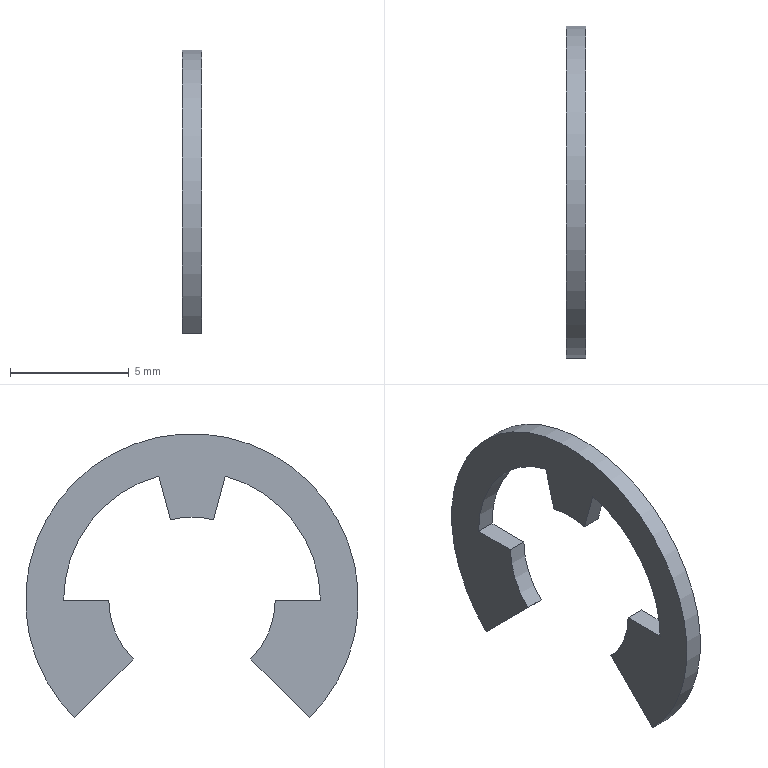Part | STEP file | 0217_Z_SCCG8-55-2 | 1 solid | 14 faces | box 0.8 x 14 x 11.95 mm | volume 51.564 mm3 | plane 8 | cylinder 6 | commonest cylinder face diameters 7 x3 10.8 x2 14 x1
STEP:
#1=CARTESIAN_POINT('',(0.,0.,0.));
#2=DIRECTION('',(0.,0.,1.));
#3=DIRECTION('',(1.,0.,0.));
#4=AXIS2_PLACEMENT_3D('',#1,#2,#3);
#5=CARTESIAN_POINT('',(3.,-2.475,-2.475));
#6=VERTEX_POINT('',#5);
#7=CARTESIAN_POINT('',(3.,-4.95,-4.95));
#8=VERTEX_POINT('',#7);
#9=CARTESIAN_POINT('',(3.,-2.475,-2.475));
#10=DIRECTION('',(0.,-0.7071,-0.7071));
#11=VECTOR('',#10,1.);
#12=LINE('',#9,#11);
#13=CARTESIAN_POINT('',(3.,0.,0.));
#14=DIRECTION('',(-1.,0.,0.));
#15=DIRECTION('',(0.,0.,1.));
#16=AXIS2_PLACEMENT_3D('',#13,#14,#15);
#17=PLANE('',#16);
#18=CARTESIAN_POINT('',(-2.475,-2.475));
#19=DIRECTION('',(-0.7071,-0.7071));
#20=VECTOR('',#19,1.);
#21=LINE('',#18,#20);
#22=(GEOMETRIC_REPRESENTATION_CONTEXT(2)PARAMETRIC_REPRESENTATION_CONTEXT()REPRESENTATION_CONTEXT('',''));
#23=DEFINITIONAL_REPRESENTATION('',(#21),#22);
#24=PCURVE('',#17,#23);
#25=CARTESIAN_POINT('',(3.,-4.95,-4.95));
#26=DIRECTION('',(0.,0.7071,-0.7071));
#27=DIRECTION('',(0.,0.7071,0.7071));
#28=AXIS2_PLACEMENT_3D('',#25,#26,#27);
#29=PLANE('',#28);
#30=CARTESIAN_POINT('',(3.5,0.));
#31=DIRECTION('',(-1.,0.));
#32=VECTOR('',#31,1.);
#33=LINE('',#30,#32);
#34=(GEOMETRIC_REPRESENTATION_CONTEXT(2)PARAMETRIC_REPRESENTATION_CONTEXT()REPRESENTATION_CONTEXT('',''));
#35=DEFINITIONAL_REPRESENTATION('',(#33),#34);
#36=PCURVE('',#29,#35);
#37=SURFACE_CURVE('',#12,(#24,#36),.PCURVE_S1.);
#38=EDGE_CURVE('',#6,#8,#37,.T.);
#39=ORIENTED_EDGE('',*,*,#38,.F.);
#40=CARTESIAN_POINT('',(3.,-3.5,0.));
#41=VERTEX_POINT('',#40);
#42=CARTESIAN_POINT('',(3.,0.,0.));
#43=DIRECTION('',(1.,0.,0.));
#44=DIRECTION('',(0.,0.,-1.));
#45=AXIS2_PLACEMENT_3D('',#42,#43,#44);
#46=CIRCLE('',#45,3.5);
#47=CARTESIAN_POINT('',(-3.5,0.));
#48=CARTESIAN_POINT('',(-3.5,6.062));
#49=CARTESIAN_POINT('',(1.75,3.031));
#50=CARTESIAN_POINT('',(7.,0.));
#51=CARTESIAN_POINT('',(1.75,-3.031));
#52=CARTESIAN_POINT('',(-3.5,-6.062));
#53=CARTESIAN_POINT('',(-3.5,0.));
#54=(BOUNDED_CURVE()B_SPLINE_CURVE(2,(#47,#48,#49,#50,#51,#52,#53),.UNSPECIFIED.,.T.,.F.)B_SPLINE_CURVE_WITH_KNOTS((1,2,2,2,2,1),(-2.094,0.,2.094,4.189,6.283,8.378),.UNSPECIFIED.)CURVE()GEOMETRIC_REPRESENTATION_ITEM()RATIONAL_B_SPLINE_CURVE((1.,0.5,1.,0.5,1.,0.5,1.))REPRESENTATION_ITEM(''));
#55=(GEOMETRIC_REPRESENTATION_CONTEXT(2)PARAMETRIC_REPRESENTATION_CONTEXT()REPRESENTATION_CONTEXT('',''));
#56=DEFINITIONAL_REPRESENTATION('',(#54),#55);
#57=PCURVE('',#17,#56);
#58=CARTESIAN_POINT('',(3.,0.,0.));
#59=DIRECTION('',(1.,0.,0.));
#60=DIRECTION('',(0.,0.,-1.));
#61=AXIS2_PLACEMENT_3D('',#58,#59,#60);
#62=CYLINDRICAL_SURFACE('',#61,3.5);
#63=CARTESIAN_POINT('',(0.,0.));
#64=DIRECTION('',(1.,0.));
#65=VECTOR('',#64,1.);
#66=LINE('',#63,#65);
#67=(GEOMETRIC_REPRESENTATION_CONTEXT(2)PARAMETRIC_REPRESENTATION_CONTEXT()REPRESENTATION_CONTEXT('',''));
#68=DEFINITIONAL_REPRESENTATION('',(#66),#67);
#69=PCURVE('',#62,#68);
#70=SURFACE_CURVE('',#46,(#57,#69),.PCURVE_S1.);
#71=EDGE_CURVE('',#41,#6,#70,.T.);
#72=ORIENTED_EDGE('',*,*,#71,.F.);
#73=CARTESIAN_POINT('',(3.,-5.4,0.));
#74=VERTEX_POINT('',#73);
#75=CARTESIAN_POINT('',(3.,0.,0.));
#76=DIRECTION('',(0.,1.,0.));
#77=VECTOR('',#76,1.);
#78=LINE('',#75,#77);
#79=CARTESIAN_POINT('',(0.,0.));
#80=DIRECTION('',(0.,1.));
#81=VECTOR('',#80,1.);
#82=LINE('',#79,#81);
#83=(GEOMETRIC_REPRESENTATION_CONTEXT(2)PARAMETRIC_REPRESENTATION_CONTEXT()REPRESENTATION_CONTEXT('',''));
#84=DEFINITIONAL_REPRESENTATION('',(#82),#83);
#85=PCURVE('',#17,#84);
#86=CARTESIAN_POINT('',(3.,-3.5,0.));
#87=DIRECTION('',(0.,0.,1.));
#88=DIRECTION('',(1.,0.,0.));
#89=AXIS2_PLACEMENT_3D('',#86,#87,#88);
#90=PLANE('',#89);
#91=CARTESIAN_POINT('',(0.,3.5));
#92=DIRECTION('',(0.,1.));
#93=VECTOR('',#92,1.);
#94=LINE('',#91,#93);
#95=(GEOMETRIC_REPRESENTATION_CONTEXT(2)PARAMETRIC_REPRESENTATION_CONTEXT()REPRESENTATION_CONTEXT('',''));
#96=DEFINITIONAL_REPRESENTATION('',(#94),#95);
#97=PCURVE('',#90,#96);
#98=SURFACE_CURVE('',#78,(#85,#97),.PCURVE_S1.);
#99=EDGE_CURVE('',#74,#41,#98,.T.);
#100=ORIENTED_EDGE('',*,*,#99,.F.);
#101=CARTESIAN_POINT('',(3.,-1.398,5.216));
#102=VERTEX_POINT('',#101);
#103=CARTESIAN_POINT('',(3.,0.,0.));
#104=DIRECTION('',(1.,0.,0.));
#105=DIRECTION('',(0.,0.,-1.));
#106=AXIS2_PLACEMENT_3D('',#103,#104,#105);
#107=CIRCLE('',#106,5.4);
#108=CARTESIAN_POINT('',(-5.4,0.));
#109=CARTESIAN_POINT('',(-5.4,9.353));
#110=CARTESIAN_POINT('',(2.7,4.677));
#111=CARTESIAN_POINT('',(10.8,0.));
#112=CARTESIAN_POINT('',(2.7,-4.677));
#113=CARTESIAN_POINT('',(-5.4,-9.353));
#114=CARTESIAN_POINT('',(-5.4,0.));
#115=(BOUNDED_CURVE()B_SPLINE_CURVE(2,(#108,#109,#110,#111,#112,#113,#114),.UNSPECIFIED.,.T.,.F.)B_SPLINE_CURVE_WITH_KNOTS((1,2,2,2,2,1),(-2.094,0.,2.094,4.189,6.283,8.378),.UNSPECIFIED.)CURVE()GEOMETRIC_REPRESENTATION_ITEM()RATIONAL_B_SPLINE_CURVE((1.,0.5,1.,0.5,1.,0.5,1.))REPRESENTATION_ITEM(''));
#116=(GEOMETRIC_REPRESENTATION_CONTEXT(2)PARAMETRIC_REPRESENTATION_CONTEXT()REPRESENTATION_CONTEXT('',''));
#117=DEFINITIONAL_REPRESENTATION('',(#115),#116);
#118=PCURVE('',#17,#117);
#119=CARTESIAN_POINT('',(3.,0.,0.));
#120=DIRECTION('',(1.,0.,0.));
#121=DIRECTION('',(0.,0.,-1.));
#122=AXIS2_PLACEMENT_3D('',#119,#120,#121);
#123=CYLINDRICAL_SURFACE('',#122,5.4);
#124=CARTESIAN_POINT('',(0.,0.));
#125=DIRECTION('',(1.,0.));
#126=VECTOR('',#125,1.);
#127=LINE('',#124,#126);
#128=(GEOMETRIC_REPRESENTATION_CONTEXT(2)PARAMETRIC_REPRESENTATION_CONTEXT()REPRESENTATION_CONTEXT('',''));
#129=DEFINITIONAL_REPRESENTATION('',(#127),#128);
#130=PCURVE('',#123,#129);
#131=SURFACE_CURVE('',#107,(#118,#130),.PCURVE_S1.);
#132=EDGE_CURVE('',#102,#74,#131,.T.);
#133=ORIENTED_EDGE('',*,*,#132,.F.);
#134=CARTESIAN_POINT('',(3.,-0.9059,3.381));
#135=VERTEX_POINT('',#134);
#136=CARTESIAN_POINT('',(3.,-0.9059,3.381));
#137=DIRECTION('',(0.,-0.2588,0.9659));
#138=VECTOR('',#137,1.);
#139=LINE('',#136,#138);
#140=CARTESIAN_POINT('',(3.381,-0.9059));
#141=DIRECTION('',(0.9659,-0.2588));
#142=VECTOR('',#141,1.);
#143=LINE('',#140,#142);
#144=(GEOMETRIC_REPRESENTATION_CONTEXT(2)PARAMETRIC_REPRESENTATION_CONTEXT()REPRESENTATION_CONTEXT('',''));
#145=DEFINITIONAL_REPRESENTATION('',(#143),#144);
#146=PCURVE('',#17,#145);
#147=CARTESIAN_POINT('',(3.,-1.398,5.216));
#148=DIRECTION('',(0.,-0.9659,-0.2588));
#149=DIRECTION('',(0.,0.2588,-0.9659));
#150=AXIS2_PLACEMENT_3D('',#147,#148,#149);
#151=PLANE('',#150);
#152=CARTESIAN_POINT('',(1.9,0.));
#153=DIRECTION('',(-1.,0.));
#154=VECTOR('',#153,1.);
#155=LINE('',#152,#154);
#156=(GEOMETRIC_REPRESENTATION_CONTEXT(2)PARAMETRIC_REPRESENTATION_CONTEXT()REPRESENTATION_CONTEXT('',''));
#157=DEFINITIONAL_REPRESENTATION('',(#155),#156);
#158=PCURVE('',#151,#157);
#159=SURFACE_CURVE('',#139,(#146,#158),.PCURVE_S1.);
#160=EDGE_CURVE('',#135,#102,#159,.T.);
#161=ORIENTED_EDGE('',*,*,#160,.F.);
#162=CARTESIAN_POINT('',(3.,0.9059,3.381));
#163=VERTEX_POINT('',#162);
#164=CARTESIAN_POINT('',(3.,0.,0.));
#165=DIRECTION('',(1.,0.,0.));
#166=DIRECTION('',(0.,0.,-1.));
#167=AXIS2_PLACEMENT_3D('',#164,#165,#166);
#168=CIRCLE('',#167,3.5);
#169=CARTESIAN_POINT('',(-3.5,0.));
#170=CARTESIAN_POINT('',(-3.5,6.062));
#171=CARTESIAN_POINT('',(1.75,3.031));
#172=CARTESIAN_POINT('',(7.,0.));
#173=CARTESIAN_POINT('',(1.75,-3.031));
#174=CARTESIAN_POINT('',(-3.5,-6.062));
#175=CARTESIAN_POINT('',(-3.5,0.));
#176=(BOUNDED_CURVE()B_SPLINE_CURVE(2,(#169,#170,#171,#172,#173,#174,#175),.UNSPECIFIED.,.T.,.F.)B_SPLINE_CURVE_WITH_KNOTS((1,2,2,2,2,1),(-2.094,0.,2.094,4.189,6.283,8.378),.UNSPECIFIED.)CURVE()GEOMETRIC_REPRESENTATION_ITEM()RATIONAL_B_SPLINE_CURVE((1.,0.5,1.,0.5,1.,0.5,1.))REPRESENTATION_ITEM(''));
#177=(GEOMETRIC_REPRESENTATION_CONTEXT(2)PARAMETRIC_REPRESENTATION_CONTEXT()REPRESENTATION_CONTEXT('',''));
#178=DEFINITIONAL_REPRESENTATION('',(#176),#177);
#179=PCURVE('',#17,#178);
#180=CARTESIAN_POINT('',(3.,0.,0.));
#181=DIRECTION('',(1.,0.,0.));
#182=DIRECTION('',(0.,0.,-1.));
#183=AXIS2_PLACEMENT_3D('',#180,#181,#182);
#184=CYLINDRICAL_SURFACE('',#183,3.5);
#185=CARTESIAN_POINT('',(0.,0.));
#186=DIRECTION('',(1.,0.));
#187=VECTOR('',#186,1.);
#188=LINE('',#185,#187);
#189=(GEOMETRIC_REPRESENTATION_CONTEXT(2)PARAMETRIC_REPRESENTATION_CONTEXT()REPRESENTATION_CONTEXT('',''));
#190=DEFINITIONAL_REPRESENTATION('',(#188),#189);
#191=PCURVE('',#184,#190);
#192=SURFACE_CURVE('',#168,(#179,#191),.PCURVE_S1.);
#193=EDGE_CURVE('',#163,#135,#192,.T.);
#194=ORIENTED_EDGE('',*,*,#193,.F.);
#195=CARTESIAN_POINT('',(3.,1.398,5.216));
#196=VERTEX_POINT('',#195);
#197=CARTESIAN_POINT('',(3.,1.398,5.216));
#198=DIRECTION('',(0.,-0.2588,-0.9659));
#199=VECTOR('',#198,1.);
#200=LINE('',#197,#199);
#201=CARTESIAN_POINT('',(5.216,1.398));
#202=DIRECTION('',(-0.9659,-0.2588));
#203=VECTOR('',#202,1.);
#204=LINE('',#201,#203);
#205=(GEOMETRIC_REPRESENTATION_CONTEXT(2)PARAMETRIC_REPRESENTATION_CONTEXT()REPRESENTATION_CONTEXT('',''));
#206=DEFINITIONAL_REPRESENTATION('',(#204),#205);
#207=PCURVE('',#17,#206);
#208=CARTESIAN_POINT('',(3.,0.9059,3.381));
#209=DIRECTION('',(0.,0.9659,-0.2588));
#210=DIRECTION('',(0.,0.2588,0.9659));
#211=AXIS2_PLACEMENT_3D('',#208,#209,#210);
#212=PLANE('',#211);
#213=CARTESIAN_POINT('',(1.9,0.));
#214=DIRECTION('',(-1.,0.));
#215=VECTOR('',#214,1.);
#216=LINE('',#213,#215);
#217=(GEOMETRIC_REPRESENTATION_CONTEXT(2)PARAMETRIC_REPRESENTATION_CONTEXT()REPRESENTATION_CONTEXT('',''));
#218=DEFINITIONAL_REPRESENTATION('',(#216),#217);
#219=PCURVE('',#212,#218);
#220=SURFACE_CURVE('',#200,(#207,#219),.PCURVE_S1.);
#221=EDGE_CURVE('',#196,#163,#220,.T.);
#222=ORIENTED_EDGE('',*,*,#221,.F.);
#223=CARTESIAN_POINT('',(3.,5.4,0.));
#224=VERTEX_POINT('',#223);
#225=CARTESIAN_POINT('',(3.,0.,0.));
#226=DIRECTION('',(1.,0.,0.));
#227=DIRECTION('',(0.,0.,-1.));
#228=AXIS2_PLACEMENT_3D('',#225,#226,#227);
#229=CIRCLE('',#228,5.4);
#230=CARTESIAN_POINT('',(-5.4,0.));
#231=CARTESIAN_POINT('',(-5.4,9.353));
#232=CARTESIAN_POINT('',(2.7,4.677));
#233=CARTESIAN_POINT('',(10.8,0.));
#234=CARTESIAN_POINT('',(2.7,-4.677));
#235=CARTESIAN_POINT('',(-5.4,-9.353));
#236=CARTESIAN_POINT('',(-5.4,0.));
#237=(BOUNDED_CURVE()B_SPLINE_CURVE(2,(#230,#231,#232,#233,#234,#235,#236),.UNSPECIFIED.,.T.,.F.)B_SPLINE_CURVE_WITH_KNOTS((1,2,2,2,2,1),(-2.094,0.,2.094,4.189,6.283,8.378),.UNSPECIFIED.)CURVE()GEOMETRIC_REPRESENTATION_ITEM()RATIONAL_B_SPLINE_CURVE((1.,0.5,1.,0.5,1.,0.5,1.))REPRESENTATION_ITEM(''));
#238=(GEOMETRIC_REPRESENTATION_CONTEXT(2)PARAMETRIC_REPRESENTATION_CONTEXT()REPRESENTATION_CONTEXT('',''));
#239=DEFINITIONAL_REPRESENTATION('',(#237),#238);
#240=PCURVE('',#17,#239);
#241=CARTESIAN_POINT('',(3.,0.,0.));
#242=DIRECTION('',(1.,0.,0.));
#243=DIRECTION('',(0.,0.,-1.));
#244=AXIS2_PLACEMENT_3D('',#241,#242,#243);
#245=CYLINDRICAL_SURFACE('',#244,5.4);
#246=CARTESIAN_POINT('',(0.,0.));
#247=DIRECTION('',(1.,0.));
#248=VECTOR('',#247,1.);
#249=LINE('',#246,#248);
#250=(GEOMETRIC_REPRESENTATION_CONTEXT(2)PARAMETRIC_REPRESENTATION_CONTEXT()REPRESENTATION_CONTEXT('',''));
#251=DEFINITIONAL_REPRESENTATION('',(#249),#250);
#252=PCURVE('',#245,#251);
#253=SURFACE_CURVE('',#229,(#240,#252),.PCURVE_S1.);
#254=EDGE_CURVE('',#224,#196,#253,.T.);
#255=ORIENTED_EDGE('',*,*,#254,.F.);
#256=CARTESIAN_POINT('',(3.,3.5,0.));
#257=VERTEX_POINT('',#256);
#258=CARTESIAN_POINT('',(3.,0.,0.));
#259=DIRECTION('',(0.,1.,0.));
#260=VECTOR('',#259,1.);
#261=LINE('',#258,#260);
#262=CARTESIAN_POINT('',(0.,0.));
#263=DIRECTION('',(0.,1.));
#264=VECTOR('',#263,1.);
#265=LINE('',#262,#264);
#266=(GEOMETRIC_REPRESENTATION_CONTEXT(2)PARAMETRIC_REPRESENTATION_CONTEXT()REPRESENTATION_CONTEXT('',''));
#267=DEFINITIONAL_REPRESENTATION('',(#265),#266);
#268=PCURVE('',#17,#267);
#269=CARTESIAN_POINT('',(3.,5.4,0.));
#270=DIRECTION('',(0.,0.,1.));
#271=DIRECTION('',(1.,0.,0.));
#272=AXIS2_PLACEMENT_3D('',#269,#270,#271);
#273=PLANE('',#272);
#274=CARTESIAN_POINT('',(0.,-5.4));
#275=DIRECTION('',(0.,1.));
#276=VECTOR('',#275,1.);
#277=LINE('',#274,#276);
#278=(GEOMETRIC_REPRESENTATION_CONTEXT(2)PARAMETRIC_REPRESENTATION_CONTEXT()REPRESENTATION_CONTEXT('',''));
#279=DEFINITIONAL_REPRESENTATION('',(#277),#278);
#280=PCURVE('',#273,#279);
#281=SURFACE_CURVE('',#261,(#268,#280),.PCURVE_S1.);
#282=EDGE_CURVE('',#257,#224,#281,.T.);
#283=ORIENTED_EDGE('',*,*,#282,.F.);
#284=CARTESIAN_POINT('',(3.,2.475,-2.475));
#285=VERTEX_POINT('',#284);
#286=CARTESIAN_POINT('',(3.,0.,0.));
#287=DIRECTION('',(1.,0.,0.));
#288=DIRECTION('',(0.,0.,-1.));
#289=AXIS2_PLACEMENT_3D('',#286,#287,#288);
#290=CIRCLE('',#289,3.5);
#291=CARTESIAN_POINT('',(-3.5,0.));
#292=CARTESIAN_POINT('',(-3.5,6.062));
#293=CARTESIAN_POINT('',(1.75,3.031));
#294=CARTESIAN_POINT('',(7.,0.));
#295=CARTESIAN_POINT('',(1.75,-3.031));
#296=CARTESIAN_POINT('',(-3.5,-6.062));
#297=CARTESIAN_POINT('',(-3.5,0.));
#298=(BOUNDED_CURVE()B_SPLINE_CURVE(2,(#291,#292,#293,#294,#295,#296,#297),.UNSPECIFIED.,.T.,.F.)B_SPLINE_CURVE_WITH_KNOTS((1,2,2,2,2,1),(-2.094,0.,2.094,4.189,6.283,8.378),.UNSPECIFIED.)CURVE()GEOMETRIC_REPRESENTATION_ITEM()RATIONAL_B_SPLINE_CURVE((1.,0.5,1.,0.5,1.,0.5,1.))REPRESENTATION_ITEM(''));
#299=(GEOMETRIC_REPRESENTATION_CONTEXT(2)PARAMETRIC_REPRESENTATION_CONTEXT()REPRESENTATION_CONTEXT('',''));
#300=DEFINITIONAL_REPRESENTATION('',(#298),#299);
#301=PCURVE('',#17,#300);
#302=CARTESIAN_POINT('',(3.,0.,0.));
#303=DIRECTION('',(1.,0.,0.));
#304=DIRECTION('',(0.,0.,-1.));
#305=AXIS2_PLACEMENT_3D('',#302,#303,#304);
#306=CYLINDRICAL_SURFACE('',#305,3.5);
#307=CARTESIAN_POINT('',(0.,0.));
#308=DIRECTION('',(1.,0.));
#309=VECTOR('',#308,1.);
#310=LINE('',#307,#309);
#311=(GEOMETRIC_REPRESENTATION_CONTEXT(2)PARAMETRIC_REPRESENTATION_CONTEXT()REPRESENTATION_CONTEXT('',''));
#312=DEFINITIONAL_REPRESENTATION('',(#310),#311);
#313=PCURVE('',#306,#312);
#314=SURFACE_CURVE('',#290,(#301,#313),.PCURVE_S1.);
#315=EDGE_CURVE('',#285,#257,#314,.T.);
#316=ORIENTED_EDGE('',*,*,#315,.F.);
#317=CARTESIAN_POINT('',(3.,4.95,-4.95));
#318=VERTEX_POINT('',#317);
#319=CARTESIAN_POINT('',(3.,4.95,-4.95));
#320=DIRECTION('',(0.,-0.7071,0.7071));
#321=VECTOR('',#320,1.);
#322=LINE('',#319,#321);
#323=CARTESIAN_POINT('',(-4.95,4.95));
#324=DIRECTION('',(0.7071,-0.7071));
#325=VECTOR('',#324,1.);
#326=LINE('',#323,#325);
#327=(GEOMETRIC_REPRESENTATION_CONTEXT(2)PARAMETRIC_REPRESENTATION_CONTEXT()REPRESENTATION_CONTEXT('',''));
#328=DEFINITIONAL_REPRESENTATION('',(#326),#327);
#329=PCURVE('',#17,#328);
#330=CARTESIAN_POINT('',(3.,2.475,-2.475));
#331=DIRECTION('',(0.,-0.7071,-0.7071));
#332=DIRECTION('',(0.,0.7071,-0.7071));
#333=AXIS2_PLACEMENT_3D('',#330,#331,#332);
#334=PLANE('',#333);
#335=CARTESIAN_POINT('',(3.5,0.));
#336=DIRECTION('',(-1.,0.));
#337=VECTOR('',#336,1.);
#338=LINE('',#335,#337);
#339=(GEOMETRIC_REPRESENTATION_CONTEXT(2)PARAMETRIC_REPRESENTATION_CONTEXT()REPRESENTATION_CONTEXT('',''));
#340=DEFINITIONAL_REPRESENTATION('',(#338),#339);
#341=PCURVE('',#334,#340);
#342=SURFACE_CURVE('',#322,(#329,#341),.PCURVE_S1.);
#343=EDGE_CURVE('',#318,#285,#342,.T.);
#344=ORIENTED_EDGE('',*,*,#343,.F.);
#345=CARTESIAN_POINT('',(3.,0.,0.));
#346=DIRECTION('',(-1.,0.,0.));
#347=DIRECTION('',(0.,0.,-1.));
#348=AXIS2_PLACEMENT_3D('',#345,#346,#347);
#349=CIRCLE('',#348,7.);
#350=CARTESIAN_POINT('',(0.,0.));
#351=DIRECTION('',(-1.,0.));
#352=AXIS2_PLACEMENT_2D('',#350,#351);
#353=CIRCLE('',#352,7.);
#354=(GEOMETRIC_REPRESENTATION_CONTEXT(2)PARAMETRIC_REPRESENTATION_CONTEXT()REPRESENTATION_CONTEXT('',''));
#355=DEFINITIONAL_REPRESENTATION('',(#353),#354);
#356=PCURVE('',#17,#355);
#357=CARTESIAN_POINT('',(3.,0.,0.));
#358=DIRECTION('',(1.,0.,0.));
#359=DIRECTION('',(0.,0.,-1.));
#360=AXIS2_PLACEMENT_3D('',#357,#358,#359);
#361=CYLINDRICAL_SURFACE('',#360,7.);
#362=CARTESIAN_POINT('',(6.283,0.));
#363=DIRECTION('',(-1.,0.));
#364=VECTOR('',#363,1.);
#365=LINE('',#362,#364);
#366=(GEOMETRIC_REPRESENTATION_CONTEXT(2)PARAMETRIC_REPRESENTATION_CONTEXT()REPRESENTATION_CONTEXT('',''));
#367=DEFINITIONAL_REPRESENTATION('',(#365),#366);
#368=PCURVE('',#361,#367);
#369=SURFACE_CURVE('',#349,(#356,#368),.PCURVE_S1.);
#370=EDGE_CURVE('',#8,#318,#369,.T.);
#371=ORIENTED_EDGE('',*,*,#370,.F.);
#372=EDGE_LOOP('',(#39,#72,#100,#133,#161,#194,#222,#255,#283,#316,#344,#371));
#373=FACE_BOUND('',#372,.T.);
#374=ADVANCED_FACE('',(#373),#17,.F.);
#375=CARTESIAN_POINT('',(2.2,-4.95,-4.95));
#376=VERTEX_POINT('',#375);
#377=CARTESIAN_POINT('',(3.,-4.95,-4.95));
#378=DIRECTION('',(1.,0.,0.));
#379=VECTOR('',#378,1.);
#380=LINE('',#377,#379);
#381=CARTESIAN_POINT('',(5.498,0.));
#382=DIRECTION('',(0.,1.));
#383=VECTOR('',#382,1.);
#384=LINE('',#381,#383);
#385=(GEOMETRIC_REPRESENTATION_CONTEXT(2)PARAMETRIC_REPRESENTATION_CONTEXT()REPRESENTATION_CONTEXT('',''));
#386=DEFINITIONAL_REPRESENTATION('',(#384),#385);
#387=PCURVE('',#361,#386);
#388=CARTESIAN_POINT('',(0.,0.));
#389=DIRECTION('',(0.,1.));
#390=VECTOR('',#389,1.);
#391=LINE('',#388,#390);
#392=(GEOMETRIC_REPRESENTATION_CONTEXT(2)PARAMETRIC_REPRESENTATION_CONTEXT()REPRESENTATION_CONTEXT('',''));
#393=DEFINITIONAL_REPRESENTATION('',(#391),#392);
#394=PCURVE('',#29,#393);
#395=SURFACE_CURVE('',#380,(#387,#394),.PCURVE_S1.);
#396=EDGE_CURVE('',#376,#8,#395,.T.);
#397=ORIENTED_EDGE('',*,*,#396,.T.);
#398=ORIENTED_EDGE('',*,*,#370,.T.);
#399=CARTESIAN_POINT('',(2.2,4.95,-4.95));
#400=VERTEX_POINT('',#399);
#401=CARTESIAN_POINT('',(3.,4.95,-4.95));
#402=DIRECTION('',(1.,0.,0.));
#403=VECTOR('',#402,1.);
#404=LINE('',#401,#403);
#405=CARTESIAN_POINT('',(0.7854,0.));
#406=DIRECTION('',(0.,1.));
#407=VECTOR('',#406,1.);
#408=LINE('',#405,#407);
#409=(GEOMETRIC_REPRESENTATION_CONTEXT(2)PARAMETRIC_REPRESENTATION_CONTEXT()REPRESENTATION_CONTEXT('',''));
#410=DEFINITIONAL_REPRESENTATION('',(#408),#409);
#411=PCURVE('',#361,#410);
#412=CARTESIAN_POINT('',(3.5,0.));
#413=DIRECTION('',(0.,1.));
#414=VECTOR('',#413,1.);
#415=LINE('',#412,#414);
#416=(GEOMETRIC_REPRESENTATION_CONTEXT(2)PARAMETRIC_REPRESENTATION_CONTEXT()REPRESENTATION_CONTEXT('',''));
#417=DEFINITIONAL_REPRESENTATION('',(#415),#416);
#418=PCURVE('',#334,#417);
#419=SURFACE_CURVE('',#404,(#411,#418),.PCURVE_S1.);
#420=EDGE_CURVE('',#400,#318,#419,.T.);
#421=ORIENTED_EDGE('',*,*,#420,.F.);
#422=CARTESIAN_POINT('',(2.2,0.,0.));
#423=DIRECTION('',(1.,0.,0.));
#424=DIRECTION('',(0.,0.,-1.));
#425=AXIS2_PLACEMENT_3D('',#422,#423,#424);
#426=CIRCLE('',#425,7.);
#427=CARTESIAN_POINT('',(0.,-0.8));
#428=DIRECTION('',(1.,0.));
#429=VECTOR('',#428,1.);
#430=LINE('',#427,#429);
#431=(GEOMETRIC_REPRESENTATION_CONTEXT(2)PARAMETRIC_REPRESENTATION_CONTEXT()REPRESENTATION_CONTEXT('',''));
#432=DEFINITIONAL_REPRESENTATION('',(#430),#431);
#433=PCURVE('',#361,#432);
#434=CARTESIAN_POINT('',(2.2,0.,0.));
#435=DIRECTION('',(-1.,0.,0.));
#436=DIRECTION('',(0.,0.,1.));
#437=AXIS2_PLACEMENT_3D('',#434,#435,#436);
#438=PLANE('',#437);
#439=CARTESIAN_POINT('',(-7.,0.));
#440=CARTESIAN_POINT('',(-7.,12.124));
#441=CARTESIAN_POINT('',(3.5,6.062));
#442=CARTESIAN_POINT('',(14.,0.));
#443=CARTESIAN_POINT('',(3.5,-6.062));
#444=CARTESIAN_POINT('',(-7.,-12.124));
#445=CARTESIAN_POINT('',(-7.,0.));
#446=(BOUNDED_CURVE()B_SPLINE_CURVE(2,(#439,#440,#441,#442,#443,#444,#445),.UNSPECIFIED.,.T.,.F.)B_SPLINE_CURVE_WITH_KNOTS((1,2,2,2,2,1),(-2.094,0.,2.094,4.189,6.283,8.378),.UNSPECIFIED.)CURVE()GEOMETRIC_REPRESENTATION_ITEM()RATIONAL_B_SPLINE_CURVE((1.,0.5,1.,0.5,1.,0.5,1.))REPRESENTATION_ITEM(''));
#447=(GEOMETRIC_REPRESENTATION_CONTEXT(2)PARAMETRIC_REPRESENTATION_CONTEXT()REPRESENTATION_CONTEXT('',''));
#448=DEFINITIONAL_REPRESENTATION('',(#446),#447);
#449=PCURVE('',#438,#448);
#450=SURFACE_CURVE('',#426,(#433,#449),.PCURVE_S1.);
#451=EDGE_CURVE('',#400,#376,#450,.T.);
#452=ORIENTED_EDGE('',*,*,#451,.T.);
#453=EDGE_LOOP('',(#397,#398,#421,#452));
#454=FACE_BOUND('',#453,.T.);
#455=ADVANCED_FACE('',(#454),#361,.T.);
#456=ORIENTED_EDGE('',*,*,#38,.T.);
#457=ORIENTED_EDGE('',*,*,#396,.F.);
#458=CARTESIAN_POINT('',(2.2,-2.475,-2.475));
#459=VERTEX_POINT('',#458);
#460=CARTESIAN_POINT('',(2.2,-4.95,-4.95));
#461=DIRECTION('',(0.,0.7071,0.7071));
#462=VECTOR('',#461,1.);
#463=LINE('',#460,#462);
#464=CARTESIAN_POINT('',(0.,-0.8));
#465=DIRECTION('',(1.,0.));
#466=VECTOR('',#465,1.);
#467=LINE('',#464,#466);
#468=(GEOMETRIC_REPRESENTATION_CONTEXT(2)PARAMETRIC_REPRESENTATION_CONTEXT()REPRESENTATION_CONTEXT('',''));
#469=DEFINITIONAL_REPRESENTATION('',(#467),#468);
#470=PCURVE('',#29,#469);
#471=CARTESIAN_POINT('',(-4.95,-4.95));
#472=DIRECTION('',(0.7071,0.7071));
#473=VECTOR('',#472,1.);
#474=LINE('',#471,#473);
#475=(GEOMETRIC_REPRESENTATION_CONTEXT(2)PARAMETRIC_REPRESENTATION_CONTEXT()REPRESENTATION_CONTEXT('',''));
#476=DEFINITIONAL_REPRESENTATION('',(#474),#475);
#477=PCURVE('',#438,#476);
#478=SURFACE_CURVE('',#463,(#470,#477),.PCURVE_S1.);
#479=EDGE_CURVE('',#376,#459,#478,.T.);
#480=ORIENTED_EDGE('',*,*,#479,.T.);
#481=CARTESIAN_POINT('',(3.,-2.475,-2.475));
#482=DIRECTION('',(1.,0.,0.));
#483=VECTOR('',#482,1.);
#484=LINE('',#481,#483);
#485=CARTESIAN_POINT('',(3.5,0.));
#486=DIRECTION('',(0.,1.));
#487=VECTOR('',#486,1.);
#488=LINE('',#485,#487);
#489=(GEOMETRIC_REPRESENTATION_CONTEXT(2)PARAMETRIC_REPRESENTATION_CONTEXT()REPRESENTATION_CONTEXT('',''));
#490=DEFINITIONAL_REPRESENTATION('',(#488),#489);
#491=PCURVE('',#29,#490);
#492=CARTESIAN_POINT('',(5.498,0.));
#493=DIRECTION('',(0.,1.));
#494=VECTOR('',#493,1.);
#495=LINE('',#492,#494);
#496=(GEOMETRIC_REPRESENTATION_CONTEXT(2)PARAMETRIC_REPRESENTATION_CONTEXT()REPRESENTATION_CONTEXT('',''));
#497=DEFINITIONAL_REPRESENTATION('',(#495),#496);
#498=PCURVE('',#62,#497);
#499=SURFACE_CURVE('',#484,(#491,#498),.PCURVE_S1.);
#500=EDGE_CURVE('',#459,#6,#499,.T.);
#501=ORIENTED_EDGE('',*,*,#500,.T.);
#502=EDGE_LOOP('',(#456,#457,#480,#501));
#503=FACE_BOUND('',#502,.T.);
#504=ADVANCED_FACE('',(#503),#29,.T.);
#505=CARTESIAN_POINT('',(2.2,-3.5,0.));
#506=VERTEX_POINT('',#505);
#507=CARTESIAN_POINT('',(2.2,0.,0.));
#508=DIRECTION('',(1.,0.,0.));
#509=DIRECTION('',(0.,0.,-1.));
#510=AXIS2_PLACEMENT_3D('',#507,#508,#509);
#511=CIRCLE('',#510,3.5);
#512=CARTESIAN_POINT('',(0.,-0.8));
#513=DIRECTION('',(1.,0.));
#514=VECTOR('',#513,1.);
#515=LINE('',#512,#514);
#516=(GEOMETRIC_REPRESENTATION_CONTEXT(2)PARAMETRIC_REPRESENTATION_CONTEXT()REPRESENTATION_CONTEXT('',''));
#517=DEFINITIONAL_REPRESENTATION('',(#515),#516);
#518=PCURVE('',#62,#517);
#519=CARTESIAN_POINT('',(-3.5,0.));
#520=CARTESIAN_POINT('',(-3.5,6.062));
#521=CARTESIAN_POINT('',(1.75,3.031));
#522=CARTESIAN_POINT('',(7.,0.));
#523=CARTESIAN_POINT('',(1.75,-3.031));
#524=CARTESIAN_POINT('',(-3.5,-6.062));
#525=CARTESIAN_POINT('',(-3.5,0.));
#526=(BOUNDED_CURVE()B_SPLINE_CURVE(2,(#519,#520,#521,#522,#523,#524,#525),.UNSPECIFIED.,.T.,.F.)B_SPLINE_CURVE_WITH_KNOTS((1,2,2,2,2,1),(-2.094,0.,2.094,4.189,6.283,8.378),.UNSPECIFIED.)CURVE()GEOMETRIC_REPRESENTATION_ITEM()RATIONAL_B_SPLINE_CURVE((1.,0.5,1.,0.5,1.,0.5,1.))REPRESENTATION_ITEM(''));
#527=(GEOMETRIC_REPRESENTATION_CONTEXT(2)PARAMETRIC_REPRESENTATION_CONTEXT()REPRESENTATION_CONTEXT('',''));
#528=DEFINITIONAL_REPRESENTATION('',(#526),#527);
#529=PCURVE('',#438,#528);
#530=SURFACE_CURVE('',#511,(#518,#529),.PCURVE_S1.);
#531=EDGE_CURVE('',#506,#459,#530,.T.);
#532=ORIENTED_EDGE('',*,*,#531,.T.);
#533=ORIENTED_EDGE('',*,*,#500,.T.);
#534=ORIENTED_EDGE('',*,*,#71,.F.);
#535=CARTESIAN_POINT('',(3.,-3.5,0.));
#536=DIRECTION('',(-1.,0.,0.));
#537=VECTOR('',#536,1.);
#538=LINE('',#535,#537);
#539=CARTESIAN_POINT('',(4.712,0.));
#540=DIRECTION('',(0.,-1.));
#541=VECTOR('',#540,1.);
#542=LINE('',#539,#541);
#543=(GEOMETRIC_REPRESENTATION_CONTEXT(2)PARAMETRIC_REPRESENTATION_CONTEXT()REPRESENTATION_CONTEXT('',''));
#544=DEFINITIONAL_REPRESENTATION('',(#542),#543);
#545=PCURVE('',#62,#544);
#546=CARTESIAN_POINT('',(0.,0.));
#547=DIRECTION('',(-1.,0.));
#548=VECTOR('',#547,1.);
#549=LINE('',#546,#548);
#550=(GEOMETRIC_REPRESENTATION_CONTEXT(2)PARAMETRIC_REPRESENTATION_CONTEXT()REPRESENTATION_CONTEXT('',''));
#551=DEFINITIONAL_REPRESENTATION('',(#549),#550);
#552=PCURVE('',#90,#551);
#553=SURFACE_CURVE('',#538,(#545,#552),.PCURVE_S1.);
#554=EDGE_CURVE('',#41,#506,#553,.T.);
#555=ORIENTED_EDGE('',*,*,#554,.T.);
#556=EDGE_LOOP('',(#532,#533,#534,#555));
#557=FACE_BOUND('',#556,.F.);
#558=ADVANCED_FACE('',(#557),#62,.F.);
#559=ORIENTED_EDGE('',*,*,#99,.T.);
#560=ORIENTED_EDGE('',*,*,#554,.T.);
#561=CARTESIAN_POINT('',(2.2,-5.4,0.));
#562=VERTEX_POINT('',#561);
#563=CARTESIAN_POINT('',(2.2,-3.5,0.));
#564=DIRECTION('',(0.,-1.,0.));
#565=VECTOR('',#564,1.);
#566=LINE('',#563,#565);
#567=CARTESIAN_POINT('',(-0.8,0.));
#568=DIRECTION('',(0.,-1.));
#569=VECTOR('',#568,1.);
#570=LINE('',#567,#569);
#571=(GEOMETRIC_REPRESENTATION_CONTEXT(2)PARAMETRIC_REPRESENTATION_CONTEXT()REPRESENTATION_CONTEXT('',''));
#572=DEFINITIONAL_REPRESENTATION('',(#570),#571);
#573=PCURVE('',#90,#572);
#574=CARTESIAN_POINT('',(0.,-3.5));
#575=DIRECTION('',(0.,-1.));
#576=VECTOR('',#575,1.);
#577=LINE('',#574,#576);
#578=(GEOMETRIC_REPRESENTATION_CONTEXT(2)PARAMETRIC_REPRESENTATION_CONTEXT()REPRESENTATION_CONTEXT('',''));
#579=DEFINITIONAL_REPRESENTATION('',(#577),#578);
#580=PCURVE('',#438,#579);
#581=SURFACE_CURVE('',#566,(#573,#580),.PCURVE_S1.);
#582=EDGE_CURVE('',#506,#562,#581,.T.);
#583=ORIENTED_EDGE('',*,*,#582,.T.);
#584=CARTESIAN_POINT('',(3.,-5.4,0.));
#585=DIRECTION('',(1.,0.,0.));
#586=VECTOR('',#585,1.);
#587=LINE('',#584,#586);
#588=CARTESIAN_POINT('',(0.,-1.9));
#589=DIRECTION('',(1.,0.));
#590=VECTOR('',#589,1.);
#591=LINE('',#588,#590);
#592=(GEOMETRIC_REPRESENTATION_CONTEXT(2)PARAMETRIC_REPRESENTATION_CONTEXT()REPRESENTATION_CONTEXT('',''));
#593=DEFINITIONAL_REPRESENTATION('',(#591),#592);
#594=PCURVE('',#90,#593);
#595=CARTESIAN_POINT('',(4.712,0.));
#596=DIRECTION('',(0.,1.));
#597=VECTOR('',#596,1.);
#598=LINE('',#595,#597);
#599=(GEOMETRIC_REPRESENTATION_CONTEXT(2)PARAMETRIC_REPRESENTATION_CONTEXT()REPRESENTATION_CONTEXT('',''));
#600=DEFINITIONAL_REPRESENTATION('',(#598),#599);
#601=PCURVE('',#123,#600);
#602=SURFACE_CURVE('',#587,(#594,#601),.PCURVE_S1.);
#603=EDGE_CURVE('',#562,#74,#602,.T.);
#604=ORIENTED_EDGE('',*,*,#603,.T.);
#605=EDGE_LOOP('',(#559,#560,#583,#604));
#606=FACE_BOUND('',#605,.T.);
#607=ADVANCED_FACE('',(#606),#90,.T.);
#608=CARTESIAN_POINT('',(2.2,-1.398,5.216));
#609=VERTEX_POINT('',#608);
#610=CARTESIAN_POINT('',(2.2,0.,0.));
#611=DIRECTION('',(1.,0.,0.));
#612=DIRECTION('',(0.,0.,-1.));
#613=AXIS2_PLACEMENT_3D('',#610,#611,#612);
#614=CIRCLE('',#613,5.4);
#615=CARTESIAN_POINT('',(0.,-0.8));
#616=DIRECTION('',(1.,0.));
#617=VECTOR('',#616,1.);
#618=LINE('',#615,#617);
#619=(GEOMETRIC_REPRESENTATION_CONTEXT(2)PARAMETRIC_REPRESENTATION_CONTEXT()REPRESENTATION_CONTEXT('',''));
#620=DEFINITIONAL_REPRESENTATION('',(#618),#619);
#621=PCURVE('',#123,#620);
#622=CARTESIAN_POINT('',(-5.4,0.));
#623=CARTESIAN_POINT('',(-5.4,9.353));
#624=CARTESIAN_POINT('',(2.7,4.677));
#625=CARTESIAN_POINT('',(10.8,0.));
#626=CARTESIAN_POINT('',(2.7,-4.677));
#627=CARTESIAN_POINT('',(-5.4,-9.353));
#628=CARTESIAN_POINT('',(-5.4,0.));
#629=(BOUNDED_CURVE()B_SPLINE_CURVE(2,(#622,#623,#624,#625,#626,#627,#628),.UNSPECIFIED.,.T.,.F.)B_SPLINE_CURVE_WITH_KNOTS((1,2,2,2,2,1),(-2.094,0.,2.094,4.189,6.283,8.378),.UNSPECIFIED.)CURVE()GEOMETRIC_REPRESENTATION_ITEM()RATIONAL_B_SPLINE_CURVE((1.,0.5,1.,0.5,1.,0.5,1.))REPRESENTATION_ITEM(''));
#630=(GEOMETRIC_REPRESENTATION_CONTEXT(2)PARAMETRIC_REPRESENTATION_CONTEXT()REPRESENTATION_CONTEXT('',''));
#631=DEFINITIONAL_REPRESENTATION('',(#629),#630);
#632=PCURVE('',#438,#631);
#633=SURFACE_CURVE('',#614,(#621,#632),.PCURVE_S1.);
#634=EDGE_CURVE('',#609,#562,#633,.T.);
#635=ORIENTED_EDGE('',*,*,#634,.T.);
#636=ORIENTED_EDGE('',*,*,#603,.T.);
#637=ORIENTED_EDGE('',*,*,#132,.F.);
#638=CARTESIAN_POINT('',(3.,-1.398,5.216));
#639=DIRECTION('',(-1.,0.,0.));
#640=VECTOR('',#639,1.);
#641=LINE('',#638,#640);
#642=CARTESIAN_POINT('',(3.403,0.));
#643=DIRECTION('',(0.,-1.));
#644=VECTOR('',#643,1.);
#645=LINE('',#642,#644);
#646=(GEOMETRIC_REPRESENTATION_CONTEXT(2)PARAMETRIC_REPRESENTATION_CONTEXT()REPRESENTATION_CONTEXT('',''));
#647=DEFINITIONAL_REPRESENTATION('',(#645),#646);
#648=PCURVE('',#123,#647);
#649=CARTESIAN_POINT('',(0.,0.));
#650=DIRECTION('',(0.,-1.));
#651=VECTOR('',#650,1.);
#652=LINE('',#649,#651);
#653=(GEOMETRIC_REPRESENTATION_CONTEXT(2)PARAMETRIC_REPRESENTATION_CONTEXT()REPRESENTATION_CONTEXT('',''));
#654=DEFINITIONAL_REPRESENTATION('',(#652),#653);
#655=PCURVE('',#151,#654);
#656=SURFACE_CURVE('',#641,(#648,#655),.PCURVE_S1.);
#657=EDGE_CURVE('',#102,#609,#656,.T.);
#658=ORIENTED_EDGE('',*,*,#657,.T.);
#659=EDGE_LOOP('',(#635,#636,#637,#658));
#660=FACE_BOUND('',#659,.F.);
#661=ADVANCED_FACE('',(#660),#123,.F.);
#662=ORIENTED_EDGE('',*,*,#160,.T.);
#663=ORIENTED_EDGE('',*,*,#657,.T.);
#664=CARTESIAN_POINT('',(2.2,-0.9059,3.381));
#665=VERTEX_POINT('',#664);
#666=CARTESIAN_POINT('',(2.2,-1.398,5.216));
#667=DIRECTION('',(0.,0.2588,-0.9659));
#668=VECTOR('',#667,1.);
#669=LINE('',#666,#668);
#670=CARTESIAN_POINT('',(0.,-0.8));
#671=DIRECTION('',(1.,0.));
#672=VECTOR('',#671,1.);
#673=LINE('',#670,#672);
#674=(GEOMETRIC_REPRESENTATION_CONTEXT(2)PARAMETRIC_REPRESENTATION_CONTEXT()REPRESENTATION_CONTEXT('',''));
#675=DEFINITIONAL_REPRESENTATION('',(#673),#674);
#676=PCURVE('',#151,#675);
#677=CARTESIAN_POINT('',(5.216,-1.398));
#678=DIRECTION('',(-0.9659,0.2588));
#679=VECTOR('',#678,1.);
#680=LINE('',#677,#679);
#681=(GEOMETRIC_REPRESENTATION_CONTEXT(2)PARAMETRIC_REPRESENTATION_CONTEXT()REPRESENTATION_CONTEXT('',''));
#682=DEFINITIONAL_REPRESENTATION('',(#680),#681);
#683=PCURVE('',#438,#682);
#684=SURFACE_CURVE('',#669,(#676,#683),.PCURVE_S1.);
#685=EDGE_CURVE('',#609,#665,#684,.T.);
#686=ORIENTED_EDGE('',*,*,#685,.T.);
#687=CARTESIAN_POINT('',(3.,-0.9059,3.381));
#688=DIRECTION('',(1.,0.,0.));
#689=VECTOR('',#688,1.);
#690=LINE('',#687,#689);
#691=CARTESIAN_POINT('',(1.9,0.));
#692=DIRECTION('',(0.,1.));
#693=VECTOR('',#692,1.);
#694=LINE('',#691,#693);
#695=(GEOMETRIC_REPRESENTATION_CONTEXT(2)PARAMETRIC_REPRESENTATION_CONTEXT()REPRESENTATION_CONTEXT('',''));
#696=DEFINITIONAL_REPRESENTATION('',(#694),#695);
#697=PCURVE('',#151,#696);
#698=CARTESIAN_POINT('',(3.403,0.));
#699=DIRECTION('',(0.,1.));
#700=VECTOR('',#699,1.);
#701=LINE('',#698,#700);
#702=(GEOMETRIC_REPRESENTATION_CONTEXT(2)PARAMETRIC_REPRESENTATION_CONTEXT()REPRESENTATION_CONTEXT('',''));
#703=DEFINITIONAL_REPRESENTATION('',(#701),#702);
#704=PCURVE('',#184,#703);
#705=SURFACE_CURVE('',#690,(#697,#704),.PCURVE_S1.);
#706=EDGE_CURVE('',#665,#135,#705,.T.);
#707=ORIENTED_EDGE('',*,*,#706,.T.);
#708=EDGE_LOOP('',(#662,#663,#686,#707));
#709=FACE_BOUND('',#708,.T.);
#710=ADVANCED_FACE('',(#709),#151,.T.);
#711=CARTESIAN_POINT('',(2.2,0.9059,3.381));
#712=VERTEX_POINT('',#711);
#713=CARTESIAN_POINT('',(2.2,0.,0.));
#714=DIRECTION('',(1.,0.,0.));
#715=DIRECTION('',(0.,0.,-1.));
#716=AXIS2_PLACEMENT_3D('',#713,#714,#715);
#717=CIRCLE('',#716,3.5);
#718=CARTESIAN_POINT('',(0.,-0.8));
#719=DIRECTION('',(1.,0.));
#720=VECTOR('',#719,1.);
#721=LINE('',#718,#720);
#722=(GEOMETRIC_REPRESENTATION_CONTEXT(2)PARAMETRIC_REPRESENTATION_CONTEXT()REPRESENTATION_CONTEXT('',''));
#723=DEFINITIONAL_REPRESENTATION('',(#721),#722);
#724=PCURVE('',#184,#723);
#725=CARTESIAN_POINT('',(-3.5,0.));
#726=CARTESIAN_POINT('',(-3.5,6.062));
#727=CARTESIAN_POINT('',(1.75,3.031));
#728=CARTESIAN_POINT('',(7.,0.));
#729=CARTESIAN_POINT('',(1.75,-3.031));
#730=CARTESIAN_POINT('',(-3.5,-6.062));
#731=CARTESIAN_POINT('',(-3.5,0.));
#732=(BOUNDED_CURVE()B_SPLINE_CURVE(2,(#725,#726,#727,#728,#729,#730,#731),.UNSPECIFIED.,.T.,.F.)B_SPLINE_CURVE_WITH_KNOTS((1,2,2,2,2,1),(-2.094,0.,2.094,4.189,6.283,8.378),.UNSPECIFIED.)CURVE()GEOMETRIC_REPRESENTATION_ITEM()RATIONAL_B_SPLINE_CURVE((1.,0.5,1.,0.5,1.,0.5,1.))REPRESENTATION_ITEM(''));
#733=(GEOMETRIC_REPRESENTATION_CONTEXT(2)PARAMETRIC_REPRESENTATION_CONTEXT()REPRESENTATION_CONTEXT('',''));
#734=DEFINITIONAL_REPRESENTATION('',(#732),#733);
#735=PCURVE('',#438,#734);
#736=SURFACE_CURVE('',#717,(#724,#735),.PCURVE_S1.);
#737=EDGE_CURVE('',#712,#665,#736,.T.);
#738=ORIENTED_EDGE('',*,*,#737,.T.);
#739=ORIENTED_EDGE('',*,*,#706,.T.);
#740=ORIENTED_EDGE('',*,*,#193,.F.);
#741=CARTESIAN_POINT('',(3.,0.9059,3.381));
#742=DIRECTION('',(-1.,0.,0.));
#743=VECTOR('',#742,1.);
#744=LINE('',#741,#743);
#745=CARTESIAN_POINT('',(2.88,0.));
#746=DIRECTION('',(0.,-1.));
#747=VECTOR('',#746,1.);
#748=LINE('',#745,#747);
#749=(GEOMETRIC_REPRESENTATION_CONTEXT(2)PARAMETRIC_REPRESENTATION_CONTEXT()REPRESENTATION_CONTEXT('',''));
#750=DEFINITIONAL_REPRESENTATION('',(#748),#749);
#751=PCURVE('',#184,#750);
#752=CARTESIAN_POINT('',(0.,0.));
#753=DIRECTION('',(0.,-1.));
#754=VECTOR('',#753,1.);
#755=LINE('',#752,#754);
#756=(GEOMETRIC_REPRESENTATION_CONTEXT(2)PARAMETRIC_REPRESENTATION_CONTEXT()REPRESENTATION_CONTEXT('',''));
#757=DEFINITIONAL_REPRESENTATION('',(#755),#756);
#758=PCURVE('',#212,#757);
#759=SURFACE_CURVE('',#744,(#751,#758),.PCURVE_S1.);
#760=EDGE_CURVE('',#163,#712,#759,.T.);
#761=ORIENTED_EDGE('',*,*,#760,.T.);
#762=EDGE_LOOP('',(#738,#739,#740,#761));
#763=FACE_BOUND('',#762,.F.);
#764=ADVANCED_FACE('',(#763),#184,.F.);
#765=ORIENTED_EDGE('',*,*,#221,.T.);
#766=ORIENTED_EDGE('',*,*,#760,.T.);
#767=CARTESIAN_POINT('',(2.2,1.398,5.216));
#768=VERTEX_POINT('',#767);
#769=CARTESIAN_POINT('',(2.2,0.9059,3.381));
#770=DIRECTION('',(0.,0.2588,0.9659));
#771=VECTOR('',#770,1.);
#772=LINE('',#769,#771);
#773=CARTESIAN_POINT('',(0.,-0.8));
#774=DIRECTION('',(1.,0.));
#775=VECTOR('',#774,1.);
#776=LINE('',#773,#775);
#777=(GEOMETRIC_REPRESENTATION_CONTEXT(2)PARAMETRIC_REPRESENTATION_CONTEXT()REPRESENTATION_CONTEXT('',''));
#778=DEFINITIONAL_REPRESENTATION('',(#776),#777);
#779=PCURVE('',#212,#778);
#780=CARTESIAN_POINT('',(3.381,0.9059));
#781=DIRECTION('',(0.9659,0.2588));
#782=VECTOR('',#781,1.);
#783=LINE('',#780,#782);
#784=(GEOMETRIC_REPRESENTATION_CONTEXT(2)PARAMETRIC_REPRESENTATION_CONTEXT()REPRESENTATION_CONTEXT('',''));
#785=DEFINITIONAL_REPRESENTATION('',(#783),#784);
#786=PCURVE('',#438,#785);
#787=SURFACE_CURVE('',#772,(#779,#786),.PCURVE_S1.);
#788=EDGE_CURVE('',#712,#768,#787,.T.);
#789=ORIENTED_EDGE('',*,*,#788,.T.);
#790=CARTESIAN_POINT('',(3.,1.398,5.216));
#791=DIRECTION('',(1.,0.,0.));
#792=VECTOR('',#791,1.);
#793=LINE('',#790,#792);
#794=CARTESIAN_POINT('',(1.9,0.));
#795=DIRECTION('',(0.,1.));
#796=VECTOR('',#795,1.);
#797=LINE('',#794,#796);
#798=(GEOMETRIC_REPRESENTATION_CONTEXT(2)PARAMETRIC_REPRESENTATION_CONTEXT()REPRESENTATION_CONTEXT('',''));
#799=DEFINITIONAL_REPRESENTATION('',(#797),#798);
#800=PCURVE('',#212,#799);
#801=CARTESIAN_POINT('',(2.88,0.));
#802=DIRECTION('',(0.,1.));
#803=VECTOR('',#802,1.);
#804=LINE('',#801,#803);
#805=(GEOMETRIC_REPRESENTATION_CONTEXT(2)PARAMETRIC_REPRESENTATION_CONTEXT()REPRESENTATION_CONTEXT('',''));
#806=DEFINITIONAL_REPRESENTATION('',(#804),#805);
#807=PCURVE('',#245,#806);
#808=SURFACE_CURVE('',#793,(#800,#807),.PCURVE_S1.);
#809=EDGE_CURVE('',#768,#196,#808,.T.);
#810=ORIENTED_EDGE('',*,*,#809,.T.);
#811=EDGE_LOOP('',(#765,#766,#789,#810));
#812=FACE_BOUND('',#811,.T.);
#813=ADVANCED_FACE('',(#812),#212,.T.);
#814=CARTESIAN_POINT('',(2.2,5.4,0.));
#815=VERTEX_POINT('',#814);
#816=CARTESIAN_POINT('',(2.2,0.,0.));
#817=DIRECTION('',(1.,0.,0.));
#818=DIRECTION('',(0.,0.,-1.));
#819=AXIS2_PLACEMENT_3D('',#816,#817,#818);
#820=CIRCLE('',#819,5.4);
#821=CARTESIAN_POINT('',(0.,-0.8));
#822=DIRECTION('',(1.,0.));
#823=VECTOR('',#822,1.);
#824=LINE('',#821,#823);
#825=(GEOMETRIC_REPRESENTATION_CONTEXT(2)PARAMETRIC_REPRESENTATION_CONTEXT()REPRESENTATION_CONTEXT('',''));
#826=DEFINITIONAL_REPRESENTATION('',(#824),#825);
#827=PCURVE('',#245,#826);
#828=CARTESIAN_POINT('',(-5.4,0.));
#829=CARTESIAN_POINT('',(-5.4,9.353));
#830=CARTESIAN_POINT('',(2.7,4.677));
#831=CARTESIAN_POINT('',(10.8,0.));
#832=CARTESIAN_POINT('',(2.7,-4.677));
#833=CARTESIAN_POINT('',(-5.4,-9.353));
#834=CARTESIAN_POINT('',(-5.4,0.));
#835=(BOUNDED_CURVE()B_SPLINE_CURVE(2,(#828,#829,#830,#831,#832,#833,#834),.UNSPECIFIED.,.T.,.F.)B_SPLINE_CURVE_WITH_KNOTS((1,2,2,2,2,1),(-2.094,0.,2.094,4.189,6.283,8.378),.UNSPECIFIED.)CURVE()GEOMETRIC_REPRESENTATION_ITEM()RATIONAL_B_SPLINE_CURVE((1.,0.5,1.,0.5,1.,0.5,1.))REPRESENTATION_ITEM(''));
#836=(GEOMETRIC_REPRESENTATION_CONTEXT(2)PARAMETRIC_REPRESENTATION_CONTEXT()REPRESENTATION_CONTEXT('',''));
#837=DEFINITIONAL_REPRESENTATION('',(#835),#836);
#838=PCURVE('',#438,#837);
#839=SURFACE_CURVE('',#820,(#827,#838),.PCURVE_S1.);
#840=EDGE_CURVE('',#815,#768,#839,.T.);
#841=ORIENTED_EDGE('',*,*,#840,.T.);
#842=ORIENTED_EDGE('',*,*,#809,.T.);
#843=ORIENTED_EDGE('',*,*,#254,.F.);
#844=CARTESIAN_POINT('',(3.,5.4,0.));
#845=DIRECTION('',(-1.,0.,0.));
#846=VECTOR('',#845,1.);
#847=LINE('',#844,#846);
#848=CARTESIAN_POINT('',(1.571,0.));
#849=DIRECTION('',(0.,-1.));
#850=VECTOR('',#849,1.);
#851=LINE('',#848,#850);
#852=(GEOMETRIC_REPRESENTATION_CONTEXT(2)PARAMETRIC_REPRESENTATION_CONTEXT()REPRESENTATION_CONTEXT('',''));
#853=DEFINITIONAL_REPRESENTATION('',(#851),#852);
#854=PCURVE('',#245,#853);
#855=CARTESIAN_POINT('',(0.,0.));
#856=DIRECTION('',(-1.,0.));
#857=VECTOR('',#856,1.);
#858=LINE('',#855,#857);
#859=(GEOMETRIC_REPRESENTATION_CONTEXT(2)PARAMETRIC_REPRESENTATION_CONTEXT()REPRESENTATION_CONTEXT('',''));
#860=DEFINITIONAL_REPRESENTATION('',(#858),#859);
#861=PCURVE('',#273,#860);
#862=SURFACE_CURVE('',#847,(#854,#861),.PCURVE_S1.);
#863=EDGE_CURVE('',#224,#815,#862,.T.);
#864=ORIENTED_EDGE('',*,*,#863,.T.);
#865=EDGE_LOOP('',(#841,#842,#843,#864));
#866=FACE_BOUND('',#865,.F.);
#867=ADVANCED_FACE('',(#866),#245,.F.);
#868=ORIENTED_EDGE('',*,*,#282,.T.);
#869=ORIENTED_EDGE('',*,*,#863,.T.);
#870=CARTESIAN_POINT('',(2.2,3.5,0.));
#871=VERTEX_POINT('',#870);
#872=CARTESIAN_POINT('',(2.2,5.4,0.));
#873=DIRECTION('',(0.,-1.,0.));
#874=VECTOR('',#873,1.);
#875=LINE('',#872,#874);
#876=CARTESIAN_POINT('',(-0.8,0.));
#877=DIRECTION('',(0.,-1.));
#878=VECTOR('',#877,1.);
#879=LINE('',#876,#878);
#880=(GEOMETRIC_REPRESENTATION_CONTEXT(2)PARAMETRIC_REPRESENTATION_CONTEXT()REPRESENTATION_CONTEXT('',''));
#881=DEFINITIONAL_REPRESENTATION('',(#879),#880);
#882=PCURVE('',#273,#881);
#883=CARTESIAN_POINT('',(0.,5.4));
#884=DIRECTION('',(0.,-1.));
#885=VECTOR('',#884,1.);
#886=LINE('',#883,#885);
#887=(GEOMETRIC_REPRESENTATION_CONTEXT(2)PARAMETRIC_REPRESENTATION_CONTEXT()REPRESENTATION_CONTEXT('',''));
#888=DEFINITIONAL_REPRESENTATION('',(#886),#887);
#889=PCURVE('',#438,#888);
#890=SURFACE_CURVE('',#875,(#882,#889),.PCURVE_S1.);
#891=EDGE_CURVE('',#815,#871,#890,.T.);
#892=ORIENTED_EDGE('',*,*,#891,.T.);
#893=CARTESIAN_POINT('',(3.,3.5,0.));
#894=DIRECTION('',(1.,0.,0.));
#895=VECTOR('',#894,1.);
#896=LINE('',#893,#895);
#897=CARTESIAN_POINT('',(0.,-1.9));
#898=DIRECTION('',(1.,0.));
#899=VECTOR('',#898,1.);
#900=LINE('',#897,#899);
#901=(GEOMETRIC_REPRESENTATION_CONTEXT(2)PARAMETRIC_REPRESENTATION_CONTEXT()REPRESENTATION_CONTEXT('',''));
#902=DEFINITIONAL_REPRESENTATION('',(#900),#901);
#903=PCURVE('',#273,#902);
#904=CARTESIAN_POINT('',(1.571,0.));
#905=DIRECTION('',(0.,1.));
#906=VECTOR('',#905,1.);
#907=LINE('',#904,#906);
#908=(GEOMETRIC_REPRESENTATION_CONTEXT(2)PARAMETRIC_REPRESENTATION_CONTEXT()REPRESENTATION_CONTEXT('',''));
#909=DEFINITIONAL_REPRESENTATION('',(#907),#908);
#910=PCURVE('',#306,#909);
#911=SURFACE_CURVE('',#896,(#903,#910),.PCURVE_S1.);
#912=EDGE_CURVE('',#871,#257,#911,.T.);
#913=ORIENTED_EDGE('',*,*,#912,.T.);
#914=EDGE_LOOP('',(#868,#869,#892,#913));
#915=FACE_BOUND('',#914,.T.);
#916=ADVANCED_FACE('',(#915),#273,.T.);
#917=CARTESIAN_POINT('',(2.2,2.475,-2.475));
#918=VERTEX_POINT('',#917);
#919=CARTESIAN_POINT('',(2.2,0.,0.));
#920=DIRECTION('',(1.,0.,0.));
#921=DIRECTION('',(0.,0.,-1.));
#922=AXIS2_PLACEMENT_3D('',#919,#920,#921);
#923=CIRCLE('',#922,3.5);
#924=CARTESIAN_POINT('',(0.,-0.8));
#925=DIRECTION('',(1.,0.));
#926=VECTOR('',#925,1.);
#927=LINE('',#924,#926);
#928=(GEOMETRIC_REPRESENTATION_CONTEXT(2)PARAMETRIC_REPRESENTATION_CONTEXT()REPRESENTATION_CONTEXT('',''));
#929=DEFINITIONAL_REPRESENTATION('',(#927),#928);
#930=PCURVE('',#306,#929);
#931=CARTESIAN_POINT('',(-3.5,0.));
#932=CARTESIAN_POINT('',(-3.5,6.062));
#933=CARTESIAN_POINT('',(1.75,3.031));
#934=CARTESIAN_POINT('',(7.,0.));
#935=CARTESIAN_POINT('',(1.75,-3.031));
#936=CARTESIAN_POINT('',(-3.5,-6.062));
#937=CARTESIAN_POINT('',(-3.5,0.));
#938=(BOUNDED_CURVE()B_SPLINE_CURVE(2,(#931,#932,#933,#934,#935,#936,#937),.UNSPECIFIED.,.T.,.F.)B_SPLINE_CURVE_WITH_KNOTS((1,2,2,2,2,1),(-2.094,0.,2.094,4.189,6.283,8.378),.UNSPECIFIED.)CURVE()GEOMETRIC_REPRESENTATION_ITEM()RATIONAL_B_SPLINE_CURVE((1.,0.5,1.,0.5,1.,0.5,1.))REPRESENTATION_ITEM(''));
#939=(GEOMETRIC_REPRESENTATION_CONTEXT(2)PARAMETRIC_REPRESENTATION_CONTEXT()REPRESENTATION_CONTEXT('',''));
#940=DEFINITIONAL_REPRESENTATION('',(#938),#939);
#941=PCURVE('',#438,#940);
#942=SURFACE_CURVE('',#923,(#930,#941),.PCURVE_S1.);
#943=EDGE_CURVE('',#918,#871,#942,.T.);
#944=ORIENTED_EDGE('',*,*,#943,.T.);
#945=ORIENTED_EDGE('',*,*,#912,.T.);
#946=ORIENTED_EDGE('',*,*,#315,.F.);
#947=CARTESIAN_POINT('',(3.,2.475,-2.475));
#948=DIRECTION('',(-1.,0.,0.));
#949=VECTOR('',#948,1.);
#950=LINE('',#947,#949);
#951=CARTESIAN_POINT('',(0.7854,0.));
#952=DIRECTION('',(0.,-1.));
#953=VECTOR('',#952,1.);
#954=LINE('',#951,#953);
#955=(GEOMETRIC_REPRESENTATION_CONTEXT(2)PARAMETRIC_REPRESENTATION_CONTEXT()REPRESENTATION_CONTEXT('',''));
#956=DEFINITIONAL_REPRESENTATION('',(#954),#955);
#957=PCURVE('',#306,#956);
#958=CARTESIAN_POINT('',(0.,0.));
#959=DIRECTION('',(0.,-1.));
#960=VECTOR('',#959,1.);
#961=LINE('',#958,#960);
#962=(GEOMETRIC_REPRESENTATION_CONTEXT(2)PARAMETRIC_REPRESENTATION_CONTEXT()REPRESENTATION_CONTEXT('',''));
#963=DEFINITIONAL_REPRESENTATION('',(#961),#962);
#964=PCURVE('',#334,#963);
#965=SURFACE_CURVE('',#950,(#957,#964),.PCURVE_S1.);
#966=EDGE_CURVE('',#285,#918,#965,.T.);
#967=ORIENTED_EDGE('',*,*,#966,.T.);
#968=EDGE_LOOP('',(#944,#945,#946,#967));
#969=FACE_BOUND('',#968,.F.);
#970=ADVANCED_FACE('',(#969),#306,.F.);
#971=ORIENTED_EDGE('',*,*,#343,.T.);
#972=ORIENTED_EDGE('',*,*,#966,.T.);
#973=CARTESIAN_POINT('',(2.2,2.475,-2.475));
#974=DIRECTION('',(0.,0.7071,-0.7071));
#975=VECTOR('',#974,1.);
#976=LINE('',#973,#975);
#977=CARTESIAN_POINT('',(0.,-0.8));
#978=DIRECTION('',(1.,0.));
#979=VECTOR('',#978,1.);
#980=LINE('',#977,#979);
#981=(GEOMETRIC_REPRESENTATION_CONTEXT(2)PARAMETRIC_REPRESENTATION_CONTEXT()REPRESENTATION_CONTEXT('',''));
#982=DEFINITIONAL_REPRESENTATION('',(#980),#981);
#983=PCURVE('',#334,#982);
#984=CARTESIAN_POINT('',(-2.475,2.475));
#985=DIRECTION('',(-0.7071,0.7071));
#986=VECTOR('',#985,1.);
#987=LINE('',#984,#986);
#988=(GEOMETRIC_REPRESENTATION_CONTEXT(2)PARAMETRIC_REPRESENTATION_CONTEXT()REPRESENTATION_CONTEXT('',''));
#989=DEFINITIONAL_REPRESENTATION('',(#987),#988);
#990=PCURVE('',#438,#989);
#991=SURFACE_CURVE('',#976,(#983,#990),.PCURVE_S1.);
#992=EDGE_CURVE('',#918,#400,#991,.T.);
#993=ORIENTED_EDGE('',*,*,#992,.T.);
#994=ORIENTED_EDGE('',*,*,#420,.T.);
#995=EDGE_LOOP('',(#971,#972,#993,#994));
#996=FACE_BOUND('',#995,.T.);
#997=ADVANCED_FACE('',(#996),#334,.T.);
#998=ORIENTED_EDGE('',*,*,#582,.F.);
#999=ORIENTED_EDGE('',*,*,#531,.T.);
#1000=ORIENTED_EDGE('',*,*,#479,.F.);
#1001=ORIENTED_EDGE('',*,*,#451,.F.);
#1002=ORIENTED_EDGE('',*,*,#992,.F.);
#1003=ORIENTED_EDGE('',*,*,#943,.T.);
#1004=ORIENTED_EDGE('',*,*,#891,.F.);
#1005=ORIENTED_EDGE('',*,*,#840,.T.);
#1006=ORIENTED_EDGE('',*,*,#788,.F.);
#1007=ORIENTED_EDGE('',*,*,#737,.T.);
#1008=ORIENTED_EDGE('',*,*,#685,.F.);
#1009=ORIENTED_EDGE('',*,*,#634,.T.);
#1010=EDGE_LOOP('',(#998,#999,#1000,#1001,#1002,#1003,#1004,#1005,#1006,#1007,#1008,#1009));
#1011=FACE_BOUND('',#1010,.T.);
#1012=ADVANCED_FACE('',(#1011),#438,.T.);
#1013=CLOSED_SHELL('',(#374,#455,#504,#558,#607,#661,#710,#764,#813,#867,#916,#970,#997,#1012));
#1014=MANIFOLD_SOLID_BREP('',#1013);
#1015=(LENGTH_UNIT()NAMED_UNIT(*)SI_UNIT(.MILLI.,.METRE.));
#1016=UNCERTAINTY_MEASURE_WITH_UNIT(LENGTH_MEASURE(0.0000001),#1015,'','');
#1017=(NAMED_UNIT(*)PLANE_ANGLE_UNIT()SI_UNIT($,.RADIAN.));
#1018=(NAMED_UNIT(*)SI_UNIT($,.STERADIAN.)SOLID_ANGLE_UNIT());
#1019=(GEOMETRIC_REPRESENTATION_CONTEXT(3)GLOBAL_UNCERTAINTY_ASSIGNED_CONTEXT((#1016))GLOBAL_UNIT_ASSIGNED_CONTEXT((#1015,#1017,#1018))REPRESENTATION_CONTEXT('',''));
#1020=ADVANCED_BREP_SHAPE_REPRESENTATION('',(#4,#1014),#1019);